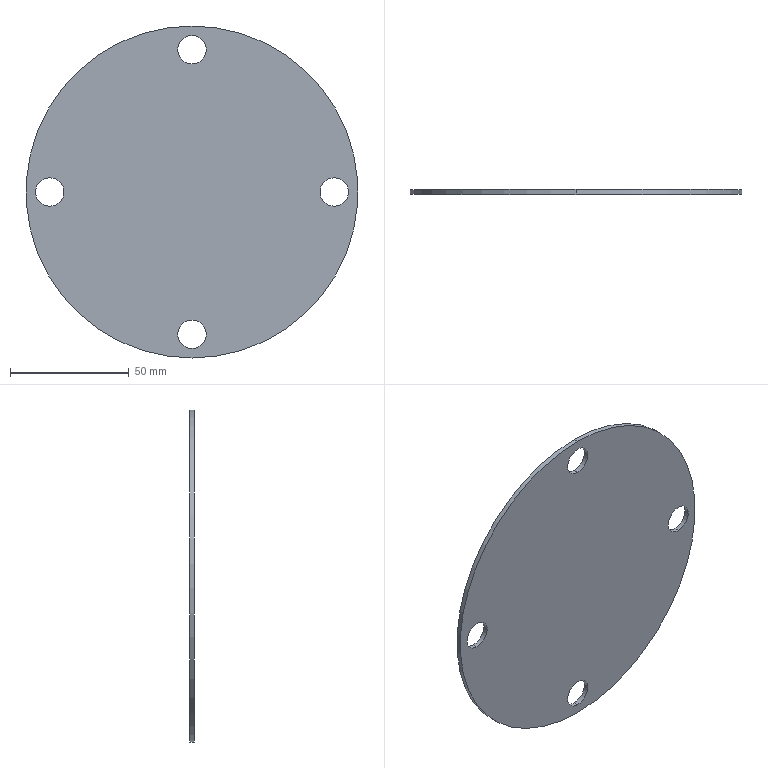Part | SolidWorks | features MirrorStock 1 | 1 solid | 12 faces | box 140 x 2 x 140 mm | volume 29883 mm3 | cylinder 10 | plane 2 | commonest cylinder face diameters 12 x8 140 x2
STEP:
#1=CARTESIAN_POINT('',(0.,0.,54.));
#2=VERTEX_POINT('',#1);
#3=CARTESIAN_POINT('',(0.,0.,66.));
#4=VERTEX_POINT('',#3);
#5=CARTESIAN_POINT('',(0.,0.,60.));
#6=DIRECTION('',(0.,-1.,0.));
#7=DIRECTION('',(0.,0.,-1.));
#8=AXIS2_PLACEMENT_3D('',#5,#6,#7);
#9=CIRCLE('',#8,6.);
#10=EDGE_CURVE('',#2,#4,#9,.T.);
#11=ORIENTED_EDGE('',*,*,#10,.T.);
#12=CARTESIAN_POINT('',(0.,2.,66.));
#13=VERTEX_POINT('',#12);
#14=CARTESIAN_POINT('',(0.,0.,66.));
#15=DIRECTION('',(0.,1.,0.));
#16=VECTOR('',#15,1000.);
#17=LINE('',#14,#16);
#18=EDGE_CURVE('',#4,#13,#17,.T.);
#19=ORIENTED_EDGE('',*,*,#18,.T.);
#20=CARTESIAN_POINT('',(0.,2.,54.));
#21=VERTEX_POINT('',#20);
#22=CARTESIAN_POINT('',(0.,2.,60.));
#23=DIRECTION('',(0.,-1.,0.));
#24=DIRECTION('',(0.,0.,-1.));
#25=AXIS2_PLACEMENT_3D('',#22,#23,#24);
#26=CIRCLE('',#25,6.);
#27=EDGE_CURVE('',#21,#13,#26,.T.);
#28=ORIENTED_EDGE('',*,*,#27,.F.);
#29=CARTESIAN_POINT('',(0.,0.,54.));
#30=DIRECTION('',(0.,1.,0.));
#31=VECTOR('',#30,1000.);
#32=LINE('',#29,#31);
#33=EDGE_CURVE('',#2,#21,#32,.T.);
#34=ORIENTED_EDGE('',*,*,#33,.F.);
#35=EDGE_LOOP('',(#11,#19,#28,#34));
#36=FACE_OUTER_BOUND('',#35,.T.);
#37=CARTESIAN_POINT('',(0.,0.,60.));
#38=DIRECTION('',(0.,1.,0.));
#39=DIRECTION('',(0.,0.,-1.));
#40=AXIS2_PLACEMENT_3D('',#37,#38,#39);
#41=CYLINDRICAL_SURFACE('',#40,6.);
#42=ADVANCED_FACE('',(#36),#41,.F.);
#43=CARTESIAN_POINT('',(60.,0.,-6.));
#44=VERTEX_POINT('',#43);
#45=CARTESIAN_POINT('',(60.,0.,6.));
#46=VERTEX_POINT('',#45);
#47=CARTESIAN_POINT('',(60.,0.,0.));
#48=DIRECTION('',(0.,-1.,0.));
#49=DIRECTION('',(0.,0.,-1.));
#50=AXIS2_PLACEMENT_3D('',#47,#48,#49);
#51=CIRCLE('',#50,6.);
#52=EDGE_CURVE('',#44,#46,#51,.T.);
#53=ORIENTED_EDGE('',*,*,#52,.T.);
#54=CARTESIAN_POINT('',(60.,2.,6.));
#55=VERTEX_POINT('',#54);
#56=CARTESIAN_POINT('',(60.,0.,6.));
#57=DIRECTION('',(0.,1.,0.));
#58=VECTOR('',#57,1000.);
#59=LINE('',#56,#58);
#60=EDGE_CURVE('',#46,#55,#59,.T.);
#61=ORIENTED_EDGE('',*,*,#60,.T.);
#62=CARTESIAN_POINT('',(60.,2.,-6.));
#63=VERTEX_POINT('',#62);
#64=CARTESIAN_POINT('',(60.,2.,0.));
#65=DIRECTION('',(0.,-1.,0.));
#66=DIRECTION('',(0.,0.,-1.));
#67=AXIS2_PLACEMENT_3D('',#64,#65,#66);
#68=CIRCLE('',#67,6.);
#69=EDGE_CURVE('',#63,#55,#68,.T.);
#70=ORIENTED_EDGE('',*,*,#69,.F.);
#71=CARTESIAN_POINT('',(60.,0.,-6.));
#72=DIRECTION('',(0.,1.,0.));
#73=VECTOR('',#72,1000.);
#74=LINE('',#71,#73);
#75=EDGE_CURVE('',#44,#63,#74,.T.);
#76=ORIENTED_EDGE('',*,*,#75,.F.);
#77=EDGE_LOOP('',(#53,#61,#70,#76));
#78=FACE_OUTER_BOUND('',#77,.T.);
#79=CARTESIAN_POINT('',(60.,0.,0.));
#80=DIRECTION('',(0.,1.,0.));
#81=DIRECTION('',(0.,0.,-1.));
#82=AXIS2_PLACEMENT_3D('',#79,#80,#81);
#83=CYLINDRICAL_SURFACE('',#82,6.);
#84=ADVANCED_FACE('',(#78),#83,.F.);
#85=CARTESIAN_POINT('',(0.,0.,-66.));
#86=VERTEX_POINT('',#85);
#87=CARTESIAN_POINT('',(0.,0.,-54.));
#88=VERTEX_POINT('',#87);
#89=CARTESIAN_POINT('',(0.,0.,-60.));
#90=DIRECTION('',(0.,-1.,0.));
#91=DIRECTION('',(0.,0.,-1.));
#92=AXIS2_PLACEMENT_3D('',#89,#90,#91);
#93=CIRCLE('',#92,6.);
#94=EDGE_CURVE('',#86,#88,#93,.T.);
#95=ORIENTED_EDGE('',*,*,#94,.T.);
#96=CARTESIAN_POINT('',(0.,2.,-54.));
#97=VERTEX_POINT('',#96);
#98=CARTESIAN_POINT('',(0.,0.,-54.));
#99=DIRECTION('',(0.,1.,0.));
#100=VECTOR('',#99,1000.);
#101=LINE('',#98,#100);
#102=EDGE_CURVE('',#88,#97,#101,.T.);
#103=ORIENTED_EDGE('',*,*,#102,.T.);
#104=CARTESIAN_POINT('',(0.,2.,-66.));
#105=VERTEX_POINT('',#104);
#106=CARTESIAN_POINT('',(0.,2.,-60.));
#107=DIRECTION('',(0.,-1.,0.));
#108=DIRECTION('',(0.,0.,-1.));
#109=AXIS2_PLACEMENT_3D('',#106,#107,#108);
#110=CIRCLE('',#109,6.);
#111=EDGE_CURVE('',#105,#97,#110,.T.);
#112=ORIENTED_EDGE('',*,*,#111,.F.);
#113=CARTESIAN_POINT('',(0.,0.,-66.));
#114=DIRECTION('',(0.,1.,0.));
#115=VECTOR('',#114,1000.);
#116=LINE('',#113,#115);
#117=EDGE_CURVE('',#86,#105,#116,.T.);
#118=ORIENTED_EDGE('',*,*,#117,.F.);
#119=EDGE_LOOP('',(#95,#103,#112,#118));
#120=FACE_OUTER_BOUND('',#119,.T.);
#121=CARTESIAN_POINT('',(0.,0.,-60.));
#122=DIRECTION('',(0.,1.,0.));
#123=DIRECTION('',(0.,0.,-1.));
#124=AXIS2_PLACEMENT_3D('',#121,#122,#123);
#125=CYLINDRICAL_SURFACE('',#124,6.);
#126=ADVANCED_FACE('',(#120),#125,.F.);
#127=CARTESIAN_POINT('',(-60.,0.,-6.));
#128=VERTEX_POINT('',#127);
#129=CARTESIAN_POINT('',(-60.,0.,6.));
#130=VERTEX_POINT('',#129);
#131=CARTESIAN_POINT('',(-60.,0.,0.));
#132=DIRECTION('',(0.,-1.,0.));
#133=DIRECTION('',(0.,0.,-1.));
#134=AXIS2_PLACEMENT_3D('',#131,#132,#133);
#135=CIRCLE('',#134,6.);
#136=EDGE_CURVE('',#128,#130,#135,.T.);
#137=ORIENTED_EDGE('',*,*,#136,.T.);
#138=CARTESIAN_POINT('',(-60.,2.,6.));
#139=VERTEX_POINT('',#138);
#140=CARTESIAN_POINT('',(-60.,0.,6.));
#141=DIRECTION('',(0.,1.,0.));
#142=VECTOR('',#141,1000.);
#143=LINE('',#140,#142);
#144=EDGE_CURVE('',#130,#139,#143,.T.);
#145=ORIENTED_EDGE('',*,*,#144,.T.);
#146=CARTESIAN_POINT('',(-60.,2.,-6.));
#147=VERTEX_POINT('',#146);
#148=CARTESIAN_POINT('',(-60.,2.,0.));
#149=DIRECTION('',(0.,-1.,0.));
#150=DIRECTION('',(0.,0.,-1.));
#151=AXIS2_PLACEMENT_3D('',#148,#149,#150);
#152=CIRCLE('',#151,6.);
#153=EDGE_CURVE('',#147,#139,#152,.T.);
#154=ORIENTED_EDGE('',*,*,#153,.F.);
#155=CARTESIAN_POINT('',(-60.,0.,-6.));
#156=DIRECTION('',(0.,1.,0.));
#157=VECTOR('',#156,1000.);
#158=LINE('',#155,#157);
#159=EDGE_CURVE('',#128,#147,#158,.T.);
#160=ORIENTED_EDGE('',*,*,#159,.F.);
#161=EDGE_LOOP('',(#137,#145,#154,#160));
#162=FACE_OUTER_BOUND('',#161,.T.);
#163=CARTESIAN_POINT('',(-60.,0.,0.));
#164=DIRECTION('',(0.,1.,0.));
#165=DIRECTION('',(0.,0.,-1.));
#166=AXIS2_PLACEMENT_3D('',#163,#164,#165);
#167=CYLINDRICAL_SURFACE('',#166,6.);
#168=ADVANCED_FACE('',(#162),#167,.F.);
#169=CARTESIAN_POINT('',(0.,2.,70.));
#170=VERTEX_POINT('',#169);
#171=CARTESIAN_POINT('',(0.,2.,-70.));
#172=VERTEX_POINT('',#171);
#173=CARTESIAN_POINT('',(0.,2.,0.));
#174=DIRECTION('',(0.,-1.,0.));
#175=DIRECTION('',(0.,0.,-1.));
#176=AXIS2_PLACEMENT_3D('',#173,#174,#175);
#177=CIRCLE('',#176,70.);
#178=EDGE_CURVE('',#170,#172,#177,.T.);
#179=ORIENTED_EDGE('',*,*,#178,.T.);
#180=CARTESIAN_POINT('',(0.,0.,-70.));
#181=VERTEX_POINT('',#180);
#182=CARTESIAN_POINT('',(0.,2.,-70.));
#183=DIRECTION('',(0.,-1.,0.));
#184=VECTOR('',#183,1000.);
#185=LINE('',#182,#184);
#186=EDGE_CURVE('',#172,#181,#185,.T.);
#187=ORIENTED_EDGE('',*,*,#186,.T.);
#188=CARTESIAN_POINT('',(0.,0.,70.));
#189=VERTEX_POINT('',#188);
#190=CARTESIAN_POINT('',(0.,0.,0.));
#191=DIRECTION('',(0.,-1.,0.));
#192=DIRECTION('',(0.,0.,-1.));
#193=AXIS2_PLACEMENT_3D('',#190,#191,#192);
#194=CIRCLE('',#193,70.);
#195=EDGE_CURVE('',#189,#181,#194,.T.);
#196=ORIENTED_EDGE('',*,*,#195,.F.);
#197=CARTESIAN_POINT('',(0.,2.,70.));
#198=DIRECTION('',(0.,-1.,0.));
#199=VECTOR('',#198,1000.);
#200=LINE('',#197,#199);
#201=EDGE_CURVE('',#170,#189,#200,.T.);
#202=ORIENTED_EDGE('',*,*,#201,.F.);
#203=EDGE_LOOP('',(#179,#187,#196,#202));
#204=FACE_OUTER_BOUND('',#203,.T.);
#205=CARTESIAN_POINT('',(0.,2.,0.));
#206=DIRECTION('',(0.,-1.,0.));
#207=DIRECTION('',(0.,0.,1.));
#208=AXIS2_PLACEMENT_3D('',#205,#206,#207);
#209=CYLINDRICAL_SURFACE('',#208,70.);
#210=ADVANCED_FACE('',(#204),#209,.T.);
#211=ORIENTED_EDGE('',*,*,#186,.F.);
#212=CARTESIAN_POINT('',(0.,2.,0.));
#213=DIRECTION('',(0.,-1.,0.));
#214=DIRECTION('',(0.,0.,-1.));
#215=AXIS2_PLACEMENT_3D('',#212,#213,#214);
#216=CIRCLE('',#215,70.);
#217=EDGE_CURVE('',#172,#170,#216,.T.);
#218=ORIENTED_EDGE('',*,*,#217,.T.);
#219=ORIENTED_EDGE('',*,*,#201,.T.);
#220=CARTESIAN_POINT('',(0.,0.,0.));
#221=DIRECTION('',(0.,-1.,0.));
#222=DIRECTION('',(0.,0.,-1.));
#223=AXIS2_PLACEMENT_3D('',#220,#221,#222);
#224=CIRCLE('',#223,70.);
#225=EDGE_CURVE('',#181,#189,#224,.T.);
#226=ORIENTED_EDGE('',*,*,#225,.F.);
#227=EDGE_LOOP('',(#211,#218,#219,#226));
#228=FACE_OUTER_BOUND('',#227,.T.);
#229=CARTESIAN_POINT('',(0.,2.,0.));
#230=DIRECTION('',(0.,-1.,0.));
#231=DIRECTION('',(0.,0.,1.));
#232=AXIS2_PLACEMENT_3D('',#229,#230,#231);
#233=CYLINDRICAL_SURFACE('',#232,70.);
#234=ADVANCED_FACE('',(#228),#233,.T.);
#235=ORIENTED_EDGE('',*,*,#27,.T.);
#236=CARTESIAN_POINT('',(0.,2.,60.));
#237=DIRECTION('',(0.,-1.,0.));
#238=DIRECTION('',(0.,0.,-1.));
#239=AXIS2_PLACEMENT_3D('',#236,#237,#238);
#240=CIRCLE('',#239,6.);
#241=EDGE_CURVE('',#13,#21,#240,.T.);
#242=ORIENTED_EDGE('',*,*,#241,.T.);
#243=EDGE_LOOP('',(#235,#242));
#244=FACE_BOUND('',#243,.T.);
#245=ORIENTED_EDGE('',*,*,#69,.T.);
#246=CARTESIAN_POINT('',(60.,2.,0.));
#247=DIRECTION('',(0.,-1.,0.));
#248=DIRECTION('',(0.,0.,-1.));
#249=AXIS2_PLACEMENT_3D('',#246,#247,#248);
#250=CIRCLE('',#249,6.);
#251=EDGE_CURVE('',#55,#63,#250,.T.);
#252=ORIENTED_EDGE('',*,*,#251,.T.);
#253=EDGE_LOOP('',(#245,#252));
#254=FACE_BOUND('',#253,.T.);
#255=ORIENTED_EDGE('',*,*,#111,.T.);
#256=CARTESIAN_POINT('',(0.,2.,-60.));
#257=DIRECTION('',(0.,-1.,0.));
#258=DIRECTION('',(0.,0.,-1.));
#259=AXIS2_PLACEMENT_3D('',#256,#257,#258);
#260=CIRCLE('',#259,6.);
#261=EDGE_CURVE('',#97,#105,#260,.T.);
#262=ORIENTED_EDGE('',*,*,#261,.T.);
#263=EDGE_LOOP('',(#255,#262));
#264=FACE_BOUND('',#263,.T.);
#265=ORIENTED_EDGE('',*,*,#153,.T.);
#266=CARTESIAN_POINT('',(-60.,2.,0.));
#267=DIRECTION('',(0.,-1.,0.));
#268=DIRECTION('',(0.,0.,-1.));
#269=AXIS2_PLACEMENT_3D('',#266,#267,#268);
#270=CIRCLE('',#269,6.);
#271=EDGE_CURVE('',#139,#147,#270,.T.);
#272=ORIENTED_EDGE('',*,*,#271,.T.);
#273=EDGE_LOOP('',(#265,#272));
#274=FACE_BOUND('',#273,.T.);
#275=ORIENTED_EDGE('',*,*,#178,.F.);
#276=ORIENTED_EDGE('',*,*,#217,.F.);
#277=EDGE_LOOP('',(#275,#276));
#278=FACE_OUTER_BOUND('',#277,.T.);
#279=CARTESIAN_POINT('',(0.,2.,0.));
#280=DIRECTION('',(0.,1.,0.));
#281=DIRECTION('',(0.,0.,-1.));
#282=AXIS2_PLACEMENT_3D('',#279,#280,#281);
#283=PLANE('',#282);
#284=ADVANCED_FACE('',(#244,#254,#264,#274,#278),#283,.T.);
#285=ORIENTED_EDGE('',*,*,#10,.F.);
#286=CARTESIAN_POINT('',(0.,0.,60.));
#287=DIRECTION('',(0.,-1.,0.));
#288=DIRECTION('',(0.,0.,-1.));
#289=AXIS2_PLACEMENT_3D('',#286,#287,#288);
#290=CIRCLE('',#289,6.);
#291=EDGE_CURVE('',#4,#2,#290,.T.);
#292=ORIENTED_EDGE('',*,*,#291,.F.);
#293=EDGE_LOOP('',(#285,#292));
#294=FACE_BOUND('',#293,.T.);
#295=ORIENTED_EDGE('',*,*,#52,.F.);
#296=CARTESIAN_POINT('',(60.,0.,0.));
#297=DIRECTION('',(0.,-1.,0.));
#298=DIRECTION('',(0.,0.,-1.));
#299=AXIS2_PLACEMENT_3D('',#296,#297,#298);
#300=CIRCLE('',#299,6.);
#301=EDGE_CURVE('',#46,#44,#300,.T.);
#302=ORIENTED_EDGE('',*,*,#301,.F.);
#303=EDGE_LOOP('',(#295,#302));
#304=FACE_BOUND('',#303,.T.);
#305=ORIENTED_EDGE('',*,*,#94,.F.);
#306=CARTESIAN_POINT('',(0.,0.,-60.));
#307=DIRECTION('',(0.,-1.,0.));
#308=DIRECTION('',(0.,0.,-1.));
#309=AXIS2_PLACEMENT_3D('',#306,#307,#308);
#310=CIRCLE('',#309,6.);
#311=EDGE_CURVE('',#88,#86,#310,.T.);
#312=ORIENTED_EDGE('',*,*,#311,.F.);
#313=EDGE_LOOP('',(#305,#312));
#314=FACE_BOUND('',#313,.T.);
#315=ORIENTED_EDGE('',*,*,#136,.F.);
#316=CARTESIAN_POINT('',(-60.,0.,0.));
#317=DIRECTION('',(0.,-1.,0.));
#318=DIRECTION('',(0.,0.,-1.));
#319=AXIS2_PLACEMENT_3D('',#316,#317,#318);
#320=CIRCLE('',#319,6.);
#321=EDGE_CURVE('',#130,#128,#320,.T.);
#322=ORIENTED_EDGE('',*,*,#321,.F.);
#323=EDGE_LOOP('',(#315,#322));
#324=FACE_BOUND('',#323,.T.);
#325=ORIENTED_EDGE('',*,*,#195,.T.);
#326=ORIENTED_EDGE('',*,*,#225,.T.);
#327=EDGE_LOOP('',(#325,#326));
#328=FACE_OUTER_BOUND('',#327,.T.);
#329=CARTESIAN_POINT('',(0.,0.,0.));
#330=DIRECTION('',(0.,1.,0.));
#331=DIRECTION('',(0.,0.,-1.));
#332=AXIS2_PLACEMENT_3D('',#329,#330,#331);
#333=PLANE('',#332);
#334=ADVANCED_FACE('',(#294,#304,#314,#324,#328),#333,.F.);
#335=ORIENTED_EDGE('',*,*,#144,.F.);
#336=ORIENTED_EDGE('',*,*,#321,.T.);
#337=ORIENTED_EDGE('',*,*,#159,.T.);
#338=ORIENTED_EDGE('',*,*,#271,.F.);
#339=EDGE_LOOP('',(#335,#336,#337,#338));
#340=FACE_OUTER_BOUND('',#339,.T.);
#341=CARTESIAN_POINT('',(-60.,0.,0.));
#342=DIRECTION('',(0.,1.,0.));
#343=DIRECTION('',(0.,0.,-1.));
#344=AXIS2_PLACEMENT_3D('',#341,#342,#343);
#345=CYLINDRICAL_SURFACE('',#344,6.);
#346=ADVANCED_FACE('',(#340),#345,.F.);
#347=ORIENTED_EDGE('',*,*,#102,.F.);
#348=ORIENTED_EDGE('',*,*,#311,.T.);
#349=ORIENTED_EDGE('',*,*,#117,.T.);
#350=ORIENTED_EDGE('',*,*,#261,.F.);
#351=EDGE_LOOP('',(#347,#348,#349,#350));
#352=FACE_OUTER_BOUND('',#351,.T.);
#353=CARTESIAN_POINT('',(0.,0.,-60.));
#354=DIRECTION('',(0.,1.,0.));
#355=DIRECTION('',(0.,0.,-1.));
#356=AXIS2_PLACEMENT_3D('',#353,#354,#355);
#357=CYLINDRICAL_SURFACE('',#356,6.);
#358=ADVANCED_FACE('',(#352),#357,.F.);
#359=ORIENTED_EDGE('',*,*,#60,.F.);
#360=ORIENTED_EDGE('',*,*,#301,.T.);
#361=ORIENTED_EDGE('',*,*,#75,.T.);
#362=ORIENTED_EDGE('',*,*,#251,.F.);
#363=EDGE_LOOP('',(#359,#360,#361,#362));
#364=FACE_OUTER_BOUND('',#363,.T.);
#365=CARTESIAN_POINT('',(60.,0.,0.));
#366=DIRECTION('',(0.,1.,0.));
#367=DIRECTION('',(0.,0.,-1.));
#368=AXIS2_PLACEMENT_3D('',#365,#366,#367);
#369=CYLINDRICAL_SURFACE('',#368,6.);
#370=ADVANCED_FACE('',(#364),#369,.F.);
#371=ORIENTED_EDGE('',*,*,#18,.F.);
#372=ORIENTED_EDGE('',*,*,#291,.T.);
#373=ORIENTED_EDGE('',*,*,#33,.T.);
#374=ORIENTED_EDGE('',*,*,#241,.F.);
#375=EDGE_LOOP('',(#371,#372,#373,#374));
#376=FACE_OUTER_BOUND('',#375,.T.);
#377=CARTESIAN_POINT('',(0.,0.,60.));
#378=DIRECTION('',(0.,1.,0.));
#379=DIRECTION('',(0.,0.,-1.));
#380=AXIS2_PLACEMENT_3D('',#377,#378,#379);
#381=CYLINDRICAL_SURFACE('',#380,6.);
#382=ADVANCED_FACE('',(#376),#381,.F.);
#383=CLOSED_SHELL('',(#42,#84,#126,#168,#210,#234,#284,#334,#346,#358,#370,#382));
#384=MANIFOLD_SOLID_BREP('',#383);
#385=CARTESIAN_POINT('',(0.,0.,0.));
#386=DIRECTION('',(0.,0.,1.));
#387=DIRECTION('',(1.,0.,0.));
#388=AXIS2_PLACEMENT_3D('',#385,#386,#387);
#389=(LENGTH_UNIT()NAMED_UNIT(*)SI_UNIT(.MILLI.,.METRE.));
#390=UNCERTAINTY_MEASURE_WITH_UNIT(LENGTH_MEASURE(0.00001),#389,'','');
#391=(NAMED_UNIT(*)PLANE_ANGLE_UNIT()SI_UNIT($,.RADIAN.));
#392=(NAMED_UNIT(*)SI_UNIT($,.STERADIAN.)SOLID_ANGLE_UNIT());
#393=(GEOMETRIC_REPRESENTATION_CONTEXT(3)GLOBAL_UNCERTAINTY_ASSIGNED_CONTEXT((#390))GLOBAL_UNIT_ASSIGNED_CONTEXT((#389,#391,#392))REPRESENTATION_CONTEXT('',''));
#394=ADVANCED_BREP_SHAPE_REPRESENTATION('',(#384,#388),#393);